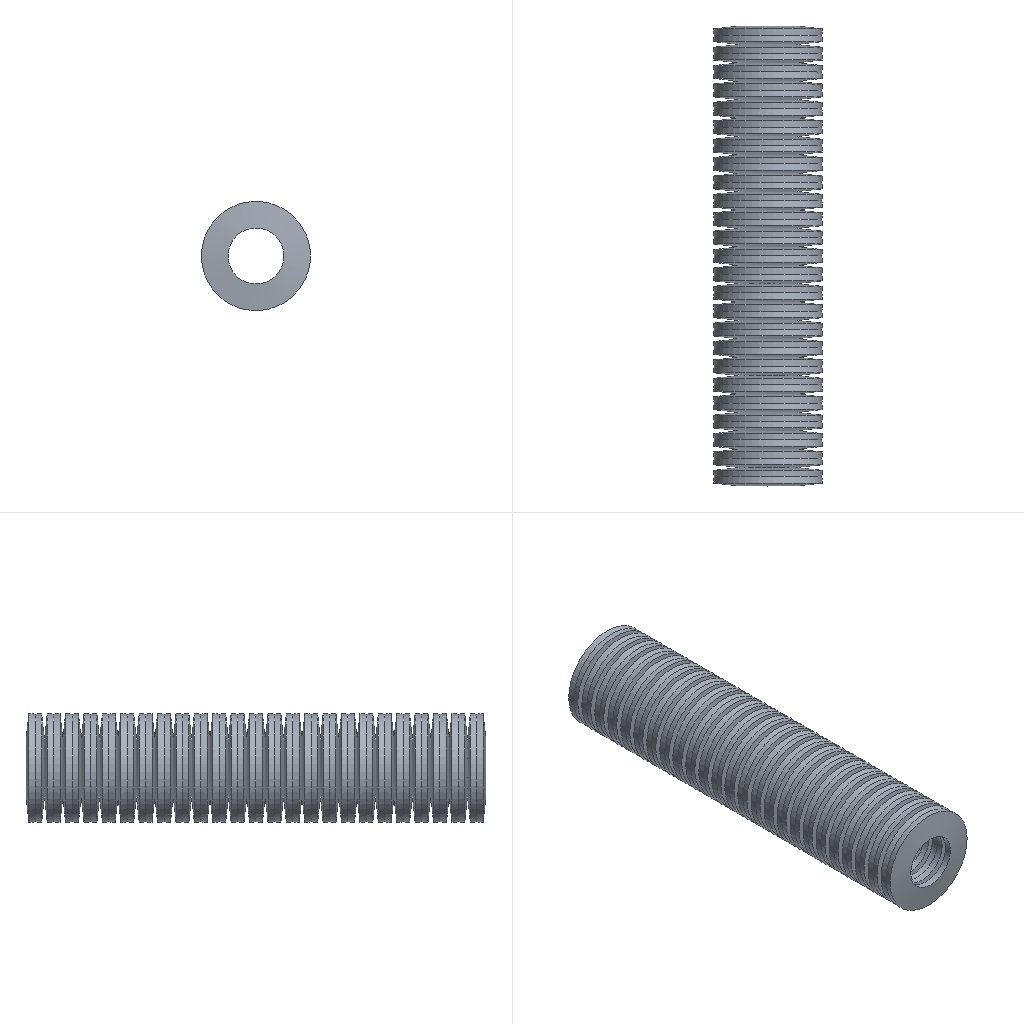Simulation study | abaqus
Set-up summary:
category,name,step,type,value,unit,region
solver,abaqus,,Abaqus/CAE 2024
units,mm-N-s-tonne (MPa),,inferred,E=206000 density=
analysis,Step-1,,static,time_period=0.24
mesh,nodes,,,129300
mesh,elements,,,18800
element_type,C3D20R,,,18800
material,Material-1,,E,206000
material,Material-1,,nu,0.3
section,Material-1,,solid section,,,_PickedSet2
bc,BC-1,initial,encastre,[dofs=ENCASTRE],,_PickedSet110
bc,BC-2,Step-1,fixed,"[dofs=rx,ry,rz,x,z n=5]",,_PickedSet113
bc,BC-2,Step-1,displacement,-1 [dofs=y],,_PickedSet113
contact,Int-1,initial,general contact,interaction=IntProp-3; friction=0.2; behavior=hard
constraint,coupling,,,1
Abaqus input file, long lists of numbers shortened, first 393 of 2027 lines:
*Heading
** Job name: deck Model name: Model-1
** Generated by: Abaqus/CAE 2024
*Preprint, echo=NO, model=NO, history=NO, contact=NO
**
** PARTS
**
*Part, name=Part-1
*Node
      1,          80.,   22.911,           0.
      2,   79.157,   13.549,           0.
** (2583 more lines like these left out)
*Element, type=C3D20R
  1,   31,   21,   17,   26,   15,    5,    1,   10,  756,  755,  754,  753,  757,  758,  759,
      760,  762,  761,  763,  764
** (750 more lines like these left out)
*Node
   2586,           0.,   27.049, 2.51052603e-15
*Nset, nset=Part-1-RefPt_, internal
2586,
*Nset, nset=_PickedSet2, internal, generate
    1,  2585,     1
*Elset, elset=_PickedSet2, internal, generate
   1,  376,    1
*Nset, nset=Set-1
    3,   19,   35,   51,   67,   83,   99,  115,  131,  147,  163,  179,  195,  211,  227,  243
  259,  275,  291,  307,  323,  339,  355,  371,  387,  403,  419,  435,  451,  467,  483,  499
** (4 more lines like these left out)
*Elset, elset=Set-1, generate
   4,  372,    8
** Section: Section-1
*Solid Section, elset=_PickedSet2, material=Material-1
,
*End Part
**
**
** ASSEMBLY
**
*Assembly, name=Assembly
**
*Instance, name=Part-1-1, part=Part-1
          0.,    -0.04861,           0.
*End Instance
**
*Instance, name=Part-1-2, part=Part-1
          0.,    27.049,           0.
          0.,    27.049,           0.,           1.,    27.049,           0.,         180.
*End Instance
**
*Instance, name=Part-1-1-lin-1-2, part=Part-1
          0.,    26.951,           0.
*End Instance
**
*Instance, name=Part-1-1-lin-1-3, part=Part-1
          0.,    53.951,           0.
*End Instance
**
*Instance, name=Part-1-1-lin-1-4, part=Part-1
          0.,    80.951,           0.
*End Instance
**
*Instance, name=Part-1-1-lin-1-5, part=Part-1
          0.,   107.951,           0.
*End Instance
**
*Instance, name=Part-1-1-lin-1-6, part=Part-1
          0.,   134.951,           0.
*End Instance
**
*Instance, name=Part-1-1-lin-1-7, part=Part-1
          0.,   161.951,           0.
*End Instance
**
*Instance, name=Part-1-1-lin-1-8, part=Part-1
          0.,   188.951,           0.
*End Instance
**
*Instance, name=Part-1-1-lin-1-9, part=Part-1
          0.,   215.951,           0.
*End Instance
**
*Instance, name=Part-1-1-lin-1-10, part=Part-1
          0.,   242.951,           0.
*End Instance
**
*Instance, name=Part-1-1-lin-1-11, part=Part-1
          0.,   269.951,           0.
*End Instance
**
*Instance, name=Part-1-1-lin-1-12, part=Part-1
          0.,   296.951,           0.
*End Instance
**
*Instance, name=Part-1-1-lin-1-13, part=Part-1
          0.,   323.951,           0.
*End Instance
**
*Instance, name=Part-1-1-lin-1-14, part=Part-1
          0.,   350.951,           0.
*End Instance
**
*Instance, name=Part-1-1-lin-1-15, part=Part-1
          0.,   377.951,           0.
*End Instance
**
*Instance, name=Part-1-1-lin-1-16, part=Part-1
          0.,   404.951,           0.
*End Instance
**
*Instance, name=Part-1-1-lin-1-17, part=Part-1
          0.,   431.951,           0.
*End Instance
**
*Instance, name=Part-1-1-lin-1-18, part=Part-1
          0.,   458.951,           0.
*End Instance
**
*Instance, name=Part-1-1-lin-1-19, part=Part-1
          0.,   485.951,           0.
*End Instance
**
*Instance, name=Part-1-1-lin-1-20, part=Part-1
          0.,   512.951,           0.
*End Instance
**
*Instance, name=Part-1-1-lin-1-21, part=Part-1
          0.,   539.951,           0.
*End Instance
**
*Instance, name=Part-1-1-lin-1-22, part=Part-1
          0.,   566.951,           0.
*End Instance
**
*Instance, name=Part-1-1-lin-1-23, part=Part-1
          0.,   593.951,           0.
*End Instance
**
*Instance, name=Part-1-1-lin-1-24, part=Part-1
          0.,   620.951,           0.
*End Instance
**
*Instance, name=Part-1-1-lin-1-25, part=Part-1
          0.,   647.951,           0.
*End Instance
**
*Instance, name=Part-1-2-lin-1-2, part=Part-1
          0.,    54.049,           0.
          0.,    54.049,           0.,           1.,    54.049,           0.,         180.
*End Instance
**
*Instance, name=Part-1-2-lin-1-3, part=Part-1
          0.,    81.049,           0.
          0.,    81.049,           0.,           1.,    81.049,           0.,         180.
*End Instance
**
*Instance, name=Part-1-2-lin-1-4, part=Part-1
          0.,   108.049,           0.
          0.,   108.049,           0.,           1.,   108.049,           0.,         180.
*End Instance
**
*Instance, name=Part-1-2-lin-1-5, part=Part-1
          0.,   135.049,           0.
          0.,   135.049,           0.,           1.,   135.049,           0.,         180.
*End Instance
**
*Instance, name=Part-1-2-lin-1-6, part=Part-1
          0.,   162.049,           0.
          0.,   162.049,           0.,           1.,   162.049,           0.,         180.
*End Instance
**
*Instance, name=Part-1-2-lin-1-7, part=Part-1
          0.,   189.049,           0.
          0.,   189.049,           0.,           1.,   189.049,           0.,         180.
*End Instance
**
*Instance, name=Part-1-2-lin-1-8, part=Part-1
          0.,   216.049,           0.
          0.,   216.049,           0.,           1.,   216.049,           0.,         180.
*End Instance
**
*Instance, name=Part-1-2-lin-1-9, part=Part-1
          0.,   243.049,           0.
          0.,   243.049,           0.,           1.,   243.049,           0.,         180.
*End Instance
**
*Instance, name=Part-1-2-lin-1-10, part=Part-1
          0.,   270.049,           0.
          0.,   270.049,           0.,           1.,   270.049,           0.,         180.
*End Instance
**
*Instance, name=Part-1-2-lin-1-11, part=Part-1
          0.,   297.049,           0.
          0.,   297.049,           0.,           1.,   297.049,           0.,         180.
*End Instance
**
*Instance, name=Part-1-2-lin-1-12, part=Part-1
          0.,   324.049,           0.
          0.,   324.049,           0.,           1.,   324.049,           0.,         180.
*End Instance
**
*Instance, name=Part-1-2-lin-1-13, part=Part-1
          0.,   351.049,           0.
          0.,   351.049,           0.,           1.,   351.049,           0.,         180.
*End Instance
**
*Instance, name=Part-1-2-lin-1-14, part=Part-1
          0.,   378.049,           0.
          0.,   378.049,           0.,           1.,   378.049,           0.,         180.
*End Instance
**
*Instance, name=Part-1-2-lin-1-15, part=Part-1
          0.,   405.049,           0.
          0.,   405.049,           0.,           1.,   405.049,           0.,         180.
*End Instance
**
*Instance, name=Part-1-2-lin-1-16, part=Part-1
          0.,   432.049,           0.
          0.,   432.049,           0.,           1.,   432.049,           0.,         180.
*End Instance
**
*Instance, name=Part-1-2-lin-1-17, part=Part-1
          0.,   459.049,           0.
          0.,   459.049,           0.,           1.,   459.049,           0.,         180.
*End Instance
**
*Instance, name=Part-1-2-lin-1-18, part=Part-1
          0.,   486.049,           0.
          0.,   486.049,           0.,           1.,   486.049,           0.,         180.
*End Instance
**
*Instance, name=Part-1-2-lin-1-19, part=Part-1
          0.,   513.049,           0.
          0.,   513.049,           0.,           1.,   513.049,           0.,         180.
*End Instance
**
*Instance, name=Part-1-2-lin-1-20, part=Part-1
          0.,   540.049,           0.
          0.,   540.049,           0.,           1.,   540.049,           0.,         180.
*End Instance
**
*Instance, name=Part-1-2-lin-1-21, part=Part-1
          0.,   567.049,           0.
          0.,   567.049,           0.,           1.,   567.049,           0.,         180.
*End Instance
**
*Instance, name=Part-1-2-lin-1-22, part=Part-1
          0.,   594.049,           0.
          0.,   594.049,           0.,           1.,   594.049,           0.,         180.
*End Instance
**
*Instance, name=Part-1-2-lin-1-23, part=Part-1
          0.,   621.049,           0.
          0.,   621.049,           0.,           1.,   621.049,           0.,         180.
*End Instance
**
*Instance, name=Part-1-2-lin-1-24, part=Part-1
          0.,   648.049,           0.
          0.,   648.049,           0.,           1.,   648.049,           0.,         180.
*End Instance
**
*Instance, name=Part-1-2-lin-1-25, part=Part-1
          0.,   675.049,           0.
          0.,   675.049,           0.,           1.,   675.049,           0.,         180.
*End Instance
**
*Nset, nset=Set-1, instance=Part-1-1-lin-1-25
 2586,
*Nset, nset=_PickedSet110, internal, instance=Part-1-2
    3,   19,   35,   51,   67,   83,   99,  115,  131,  147,  163,  179,  195,  211,  227,  243
  259,  275,  291,  307,  323,  339,  355,  371,  387,  403,  419,  435,  451,  467,  483,  499
** (4 more lines like these left out)
*Elset, elset=_PickedSet110, internal, instance=Part-1-2, generate
   4,  372,    8
*Nset, nset=_PickedSet113, internal, instance=Part-1-1-lin-1-25
 2586,
*Nset, nset=_PickedSet118, internal, instance=Part-1-2
    3,   19,   35,   51,   67,   83,   99,  115,  131,  147,  163,  179,  195,  211,  227,  243
  259,  275,  291,  307,  323,  339,  355,  371,  387,  403,  419,  435,  451,  467,  483,  499
** (4 more lines like these left out)
*Elset, elset=_PickedSet118, internal, instance=Part-1-2, generate
   4,  372,    8
*Nset, nset=_PickedSet119, internal, instance=Part-1-2
 2586,
*Nset, nset=_PickedSet120, internal, instance=Part-1-1-lin-1-25
    3,   19,   35,   51,   67,   83,   99,  115,  131,  147,  163,  179,  195,  211,  227,  243
  259,  275,  291,  307,  323,  339,  355,  371,  387,  403,  419,  435,  451,  467,  483,  499
** (4 more lines like these left out)
*Elset, elset=_PickedSet120, internal, instance=Part-1-1-lin-1-25, generate
   4,  372,    8
*Nset, nset=_PickedSet121, internal, instance=Part-1-1-lin-1-25
 2586,
*Surface, type=NODE, name=_PickedSet120_CNS_, internal
_PickedSet120, 1.
** Constraint: Constraint-2
*Coupling, constraint name=Constraint-2, ref node=_PickedSet121, surface=_PickedSet120_CNS_
*Kinematic
*Elset, elset=__Int-1_gcs0_1_S4, internal, instance=Part-1-1, generate
   1,  369,    8
*Elset, elset=__Int-1_gcs0_1_S5, internal, instance=Part-1-1, generate
   7,  375,    8
*Elset, elset=__Int-1_gcs0_1_S3, internal, instance=Part-1-1, generate
   8,  376,    8
*Surface, type=ELEMENT, name=_Int-1_gcs0_1, internal
__Int-1_gcs0_1_S4, S4
__Int-1_gcs0_1_S5, S5
__Int-1_gcs0_1_S3, S3
*Elset, elset=__Int-1_gcs0_2_S5, internal, instance=Part-1-1
   2,   4,   5,   6,  10,  12,  13,  14,  18,  20,  21,  22,  26,  28,  29,  30
  34,  36,  37,  38,  42,  44,  45,  46,  50,  52,  53,  54,  58,  60,  61,  62
** (10 more lines like these left out)
*Elset, elset=__Int-1_gcs0_2_S6, internal, instance=Part-1-1, generate
   8,  376,    8
*Surface, type=ELEMENT, name=_Int-1_gcs0_2, internal
__Int-1_gcs0_2_S5, S5
__Int-1_gcs0_2_S6, S6
*Elset, elset=__Int-1_gcs0_3_S4, internal, instance=Part-1-1, generate
   4,  372,    8
*Surface, type=ELEMENT, name=_Int-1_gcs0_3, internal
__Int-1_gcs0_3_S4, S4
*Elset, elset=__Int-1_gcs0_4_S5, internal, instance=Part-1-1, generate
   1,  369,    8
*Elset, elset=__Int-1_gcs0_4_S3, internal, instance=Part-1-1
   2,   4,   5,   6,  10,  12,  13,  14,  18,  20,  21,  22,  26,  28,  29,  30
  34,  36,  37,  38,  42,  44,  45,  46,  50,  52,  53,  54,  58,  60,  61,  62
** (10 more lines like these left out)
*Surface, type=ELEMENT, name=_Int-1_gcs0_4, internal
__Int-1_gcs0_4_S5, S5
__Int-1_gcs0_4_S3, S3
*Elset, elset=__Int-1_gcs0_5_S4, internal, instance=Part-1-2, generate
   1,  369,    8
*Elset, elset=__Int-1_gcs0_5_S5, internal, instance=Part-1-2, generate
   7,  375,    8
*Elset, elset=__Int-1_gcs0_5_S3, internal, instance=Part-1-2, generate
   8,  376,    8
*Surface, type=ELEMENT, name=_Int-1_gcs0_5, internal
__Int-1_gcs0_5_S4, S4
__Int-1_gcs0_5_S5, S5
__Int-1_gcs0_5_S3, S3
*Elset, elset=__Int-1_gcs0_6_S5, internal, instance=Part-1-2
   2,   4,   5,   6,  10,  12,  13,  14,  18,  20,  21,  22,  26,  28,  29,  30
  34,  36,  37,  38,  42,  44,  45,  46,  50,  52,  53,  54,  58,  60,  61,  62
** (10 more lines like these left out)
*Elset, elset=__Int-1_gcs0_6_S6, internal, instance=Part-1-2, generate
   8,  376,    8
*Surface, type=ELEMENT, name=_Int-1_gcs0_6, internal
__Int-1_gcs0_6_S5, S5
__Int-1_gcs0_6_S6, S6
*Elset, elset=__Int-1_gcs0_7_S4, internal, instance=Part-1-2, generate
   4,  372,    8
*Surface, type=ELEMENT, name=_Int-1_gcs0_7, internal
__Int-1_gcs0_7_S4, S4
*Elset, elset=__Int-1_gcs0_8_S5, internal, instance=Part-1-2, generate
   1,  369,    8
*Elset, elset=__Int-1_gcs0_8_S3, internal, instance=Part-1-2
   2,   4,   5,   6,  10,  12,  13,  14,  18,  20,  21,  22,  26,  28,  29,  30
  34,  36,  37,  38,  42,  44,  45,  46,  50,  52,  53,  54,  58,  60,  61,  62
** (10 more lines like these left out)
*Surface, type=ELEMENT, name=_Int-1_gcs0_8, internal
__Int-1_gcs0_8_S5, S5
__Int-1_gcs0_8_S3, S3
*Elset, elset=__Int-1_gcs0_9_S4, internal, instance=Part-1-1-lin-1-2, generate
   1,  369,    8
*Elset, elset=__Int-1_gcs0_9_S5, internal, instance=Part-1-1-lin-1-2, generate
   7,  375,    8
*Elset, elset=__Int-1_gcs0_9_S3, internal, instance=Part-1-1-lin-1-2, generate
   8,  376,    8
*Surface, type=ELEMENT, name=_Int-1_gcs0_9, internal
__Int-1_gcs0_9_S4, S4
__Int-1_gcs0_9_S5, S5
__Int-1_gcs0_9_S3, S3
*Elset, elset=__Int-1_gcs0_10_S5, internal, instance=Part-1-1-lin-1-2
   2,   4,   5,   6,  10,  12,  13,  14,  18,  20,  21,  22,  26,  28,  29,  30
  34,  36,  37,  38,  42,  44,  45,  46,  50,  52,  53,  54,  58,  60,  61,  62
** (10 more lines like these left out)
*Elset, elset=__Int-1_gcs0_10_S6, internal, instance=Part-1-1-lin-1-2, generate
   8,  376,    8
*Surface, type=ELEMENT, name=_Int-1_gcs0_10, internal
__Int-1_gcs0_10_S5, S5
__Int-1_gcs0_10_S6, S6
*Elset, elset=__Int-1_gcs0_11_S4, internal, instance=Part-1-1-lin-1-2, generate
   4,  372,    8
*Surface, type=ELEMENT, name=_Int-1_gcs0_11, internal
__Int-1_gcs0_11_S4, S4
*Elset, elset=__Int-1_gcs0_12_S5, internal, instance=Part-1-1-lin-1-2, generate
   1,  369,    8
*Elset, elset=__Int-1_gcs0_12_S3, internal, instance=Part-1-1-lin-1-2
   2,   4,   5,   6,  10,  12,  13,  14,  18,  20,  21,  22,  26,  28,  29,  30
  34,  36,  37,  38,  42,  44,  45,  46,  50,  52,  53,  54,  58,  60,  61,  62
** (10 more lines like these left out)
*Surface, type=ELEMENT, name=_Int-1_gcs0_12, internal
__Int-1_gcs0_12_S5, S5
__Int-1_gcs0_12_S3, S3
*Elset, elset=__Int-1_gcs0_13_S4, internal, instance=Part-1-1-lin-1-3, generate
Last 640 lines:
   7,  375,    8
*Elset, elset=__Int-1_gcs0_137_S3, internal, instance=Part-1-2-lin-1-10, generate
   8,  376,    8
*Surface, type=ELEMENT, name=_Int-1_gcs0_137, internal
__Int-1_gcs0_137_S4, S4
__Int-1_gcs0_137_S5, S5
__Int-1_gcs0_137_S3, S3
*Elset, elset=__Int-1_gcs0_138_S5, internal, instance=Part-1-2-lin-1-10
   2,   4,   5,   6,  10,  12,  13,  14,  18,  20,  21,  22,  26,  28,  29,  30
  34,  36,  37,  38,  42,  44,  45,  46,  50,  52,  53,  54,  58,  60,  61,  62
** (10 more lines like these left out)
*Elset, elset=__Int-1_gcs0_138_S6, internal, instance=Part-1-2-lin-1-10, generate
   8,  376,    8
*Surface, type=ELEMENT, name=_Int-1_gcs0_138, internal
__Int-1_gcs0_138_S5, S5
__Int-1_gcs0_138_S6, S6
*Elset, elset=__Int-1_gcs0_139_S4, internal, instance=Part-1-2-lin-1-10, generate
   4,  372,    8
*Surface, type=ELEMENT, name=_Int-1_gcs0_139, internal
__Int-1_gcs0_139_S4, S4
*Elset, elset=__Int-1_gcs0_140_S5, internal, instance=Part-1-2-lin-1-10, generate
   1,  369,    8
*Elset, elset=__Int-1_gcs0_140_S3, internal, instance=Part-1-2-lin-1-10
   2,   4,   5,   6,  10,  12,  13,  14,  18,  20,  21,  22,  26,  28,  29,  30
  34,  36,  37,  38,  42,  44,  45,  46,  50,  52,  53,  54,  58,  60,  61,  62
** (10 more lines like these left out)
*Surface, type=ELEMENT, name=_Int-1_gcs0_140, internal
__Int-1_gcs0_140_S5, S5
__Int-1_gcs0_140_S3, S3
*Elset, elset=__Int-1_gcs0_141_S4, internal, instance=Part-1-2-lin-1-11, generate
   1,  369,    8
*Elset, elset=__Int-1_gcs0_141_S5, internal, instance=Part-1-2-lin-1-11, generate
   7,  375,    8
*Elset, elset=__Int-1_gcs0_141_S3, internal, instance=Part-1-2-lin-1-11, generate
   8,  376,    8
*Surface, type=ELEMENT, name=_Int-1_gcs0_141, internal
__Int-1_gcs0_141_S4, S4
__Int-1_gcs0_141_S5, S5
__Int-1_gcs0_141_S3, S3
*Elset, elset=__Int-1_gcs0_142_S5, internal, instance=Part-1-2-lin-1-11
   2,   4,   5,   6,  10,  12,  13,  14,  18,  20,  21,  22,  26,  28,  29,  30
  34,  36,  37,  38,  42,  44,  45,  46,  50,  52,  53,  54,  58,  60,  61,  62
** (10 more lines like these left out)
*Elset, elset=__Int-1_gcs0_142_S6, internal, instance=Part-1-2-lin-1-11, generate
   8,  376,    8
*Surface, type=ELEMENT, name=_Int-1_gcs0_142, internal
__Int-1_gcs0_142_S5, S5
__Int-1_gcs0_142_S6, S6
*Elset, elset=__Int-1_gcs0_143_S4, internal, instance=Part-1-2-lin-1-11, generate
   4,  372,    8
*Surface, type=ELEMENT, name=_Int-1_gcs0_143, internal
__Int-1_gcs0_143_S4, S4
*Elset, elset=__Int-1_gcs0_144_S5, internal, instance=Part-1-2-lin-1-11, generate
   1,  369,    8
*Elset, elset=__Int-1_gcs0_144_S3, internal, instance=Part-1-2-lin-1-11
   2,   4,   5,   6,  10,  12,  13,  14,  18,  20,  21,  22,  26,  28,  29,  30
  34,  36,  37,  38,  42,  44,  45,  46,  50,  52,  53,  54,  58,  60,  61,  62
** (10 more lines like these left out)
*Surface, type=ELEMENT, name=_Int-1_gcs0_144, internal
__Int-1_gcs0_144_S5, S5
__Int-1_gcs0_144_S3, S3
*Elset, elset=__Int-1_gcs0_145_S4, internal, instance=Part-1-2-lin-1-12, generate
   1,  369,    8
*Elset, elset=__Int-1_gcs0_145_S5, internal, instance=Part-1-2-lin-1-12, generate
   7,  375,    8
*Elset, elset=__Int-1_gcs0_145_S3, internal, instance=Part-1-2-lin-1-12, generate
   8,  376,    8
*Surface, type=ELEMENT, name=_Int-1_gcs0_145, internal
__Int-1_gcs0_145_S4, S4
__Int-1_gcs0_145_S5, S5
__Int-1_gcs0_145_S3, S3
*Elset, elset=__Int-1_gcs0_146_S5, internal, instance=Part-1-2-lin-1-12
   2,   4,   5,   6,  10,  12,  13,  14,  18,  20,  21,  22,  26,  28,  29,  30
  34,  36,  37,  38,  42,  44,  45,  46,  50,  52,  53,  54,  58,  60,  61,  62
** (10 more lines like these left out)
*Elset, elset=__Int-1_gcs0_146_S6, internal, instance=Part-1-2-lin-1-12, generate
   8,  376,    8
*Surface, type=ELEMENT, name=_Int-1_gcs0_146, internal
__Int-1_gcs0_146_S5, S5
__Int-1_gcs0_146_S6, S6
*Elset, elset=__Int-1_gcs0_147_S4, internal, instance=Part-1-2-lin-1-12, generate
   4,  372,    8
*Surface, type=ELEMENT, name=_Int-1_gcs0_147, internal
__Int-1_gcs0_147_S4, S4
*Elset, elset=__Int-1_gcs0_148_S5, internal, instance=Part-1-2-lin-1-12, generate
   1,  369,    8
*Elset, elset=__Int-1_gcs0_148_S3, internal, instance=Part-1-2-lin-1-12
   2,   4,   5,   6,  10,  12,  13,  14,  18,  20,  21,  22,  26,  28,  29,  30
  34,  36,  37,  38,  42,  44,  45,  46,  50,  52,  53,  54,  58,  60,  61,  62
** (10 more lines like these left out)
*Surface, type=ELEMENT, name=_Int-1_gcs0_148, internal
__Int-1_gcs0_148_S5, S5
__Int-1_gcs0_148_S3, S3
*Elset, elset=__Int-1_gcs0_149_S4, internal, instance=Part-1-2-lin-1-13, generate
   1,  369,    8
*Elset, elset=__Int-1_gcs0_149_S5, internal, instance=Part-1-2-lin-1-13, generate
   7,  375,    8
*Elset, elset=__Int-1_gcs0_149_S3, internal, instance=Part-1-2-lin-1-13, generate
   8,  376,    8
*Surface, type=ELEMENT, name=_Int-1_gcs0_149, internal
__Int-1_gcs0_149_S4, S4
__Int-1_gcs0_149_S5, S5
__Int-1_gcs0_149_S3, S3
*Elset, elset=__Int-1_gcs0_150_S5, internal, instance=Part-1-2-lin-1-13
   2,   4,   5,   6,  10,  12,  13,  14,  18,  20,  21,  22,  26,  28,  29,  30
  34,  36,  37,  38,  42,  44,  45,  46,  50,  52,  53,  54,  58,  60,  61,  62
** (10 more lines like these left out)
*Elset, elset=__Int-1_gcs0_150_S6, internal, instance=Part-1-2-lin-1-13, generate
   8,  376,    8
*Surface, type=ELEMENT, name=_Int-1_gcs0_150, internal
__Int-1_gcs0_150_S5, S5
__Int-1_gcs0_150_S6, S6
*Elset, elset=__Int-1_gcs0_151_S4, internal, instance=Part-1-2-lin-1-13, generate
   4,  372,    8
*Surface, type=ELEMENT, name=_Int-1_gcs0_151, internal
__Int-1_gcs0_151_S4, S4
*Elset, elset=__Int-1_gcs0_152_S5, internal, instance=Part-1-2-lin-1-13, generate
   1,  369,    8
*Elset, elset=__Int-1_gcs0_152_S3, internal, instance=Part-1-2-lin-1-13
   2,   4,   5,   6,  10,  12,  13,  14,  18,  20,  21,  22,  26,  28,  29,  30
  34,  36,  37,  38,  42,  44,  45,  46,  50,  52,  53,  54,  58,  60,  61,  62
** (10 more lines like these left out)
*Surface, type=ELEMENT, name=_Int-1_gcs0_152, internal
__Int-1_gcs0_152_S5, S5
__Int-1_gcs0_152_S3, S3
*Elset, elset=__Int-1_gcs0_153_S4, internal, instance=Part-1-2-lin-1-14, generate
   1,  369,    8
*Elset, elset=__Int-1_gcs0_153_S5, internal, instance=Part-1-2-lin-1-14, generate
   7,  375,    8
*Elset, elset=__Int-1_gcs0_153_S3, internal, instance=Part-1-2-lin-1-14, generate
   8,  376,    8
*Surface, type=ELEMENT, name=_Int-1_gcs0_153, internal
__Int-1_gcs0_153_S4, S4
__Int-1_gcs0_153_S5, S5
__Int-1_gcs0_153_S3, S3
*Elset, elset=__Int-1_gcs0_154_S5, internal, instance=Part-1-2-lin-1-14
   2,   4,   5,   6,  10,  12,  13,  14,  18,  20,  21,  22,  26,  28,  29,  30
  34,  36,  37,  38,  42,  44,  45,  46,  50,  52,  53,  54,  58,  60,  61,  62
** (10 more lines like these left out)
*Elset, elset=__Int-1_gcs0_154_S6, internal, instance=Part-1-2-lin-1-14, generate
   8,  376,    8
*Surface, type=ELEMENT, name=_Int-1_gcs0_154, internal
__Int-1_gcs0_154_S5, S5
__Int-1_gcs0_154_S6, S6
*Elset, elset=__Int-1_gcs0_155_S4, internal, instance=Part-1-2-lin-1-14, generate
   4,  372,    8
*Surface, type=ELEMENT, name=_Int-1_gcs0_155, internal
__Int-1_gcs0_155_S4, S4
*Elset, elset=__Int-1_gcs0_156_S5, internal, instance=Part-1-2-lin-1-14, generate
   1,  369,    8
*Elset, elset=__Int-1_gcs0_156_S3, internal, instance=Part-1-2-lin-1-14
   2,   4,   5,   6,  10,  12,  13,  14,  18,  20,  21,  22,  26,  28,  29,  30
  34,  36,  37,  38,  42,  44,  45,  46,  50,  52,  53,  54,  58,  60,  61,  62
** (10 more lines like these left out)
*Surface, type=ELEMENT, name=_Int-1_gcs0_156, internal
__Int-1_gcs0_156_S5, S5
__Int-1_gcs0_156_S3, S3
*Elset, elset=__Int-1_gcs0_157_S4, internal, instance=Part-1-2-lin-1-15, generate
   1,  369,    8
*Elset, elset=__Int-1_gcs0_157_S5, internal, instance=Part-1-2-lin-1-15, generate
   7,  375,    8
*Elset, elset=__Int-1_gcs0_157_S3, internal, instance=Part-1-2-lin-1-15, generate
   8,  376,    8
*Surface, type=ELEMENT, name=_Int-1_gcs0_157, internal
__Int-1_gcs0_157_S4, S4
__Int-1_gcs0_157_S5, S5
__Int-1_gcs0_157_S3, S3
*Elset, elset=__Int-1_gcs0_158_S5, internal, instance=Part-1-2-lin-1-15
   2,   4,   5,   6,  10,  12,  13,  14,  18,  20,  21,  22,  26,  28,  29,  30
  34,  36,  37,  38,  42,  44,  45,  46,  50,  52,  53,  54,  58,  60,  61,  62
** (10 more lines like these left out)
*Elset, elset=__Int-1_gcs0_158_S6, internal, instance=Part-1-2-lin-1-15, generate
   8,  376,    8
*Surface, type=ELEMENT, name=_Int-1_gcs0_158, internal
__Int-1_gcs0_158_S5, S5
__Int-1_gcs0_158_S6, S6
*Elset, elset=__Int-1_gcs0_159_S4, internal, instance=Part-1-2-lin-1-15, generate
   4,  372,    8
*Surface, type=ELEMENT, name=_Int-1_gcs0_159, internal
__Int-1_gcs0_159_S4, S4
*Elset, elset=__Int-1_gcs0_160_S5, internal, instance=Part-1-2-lin-1-15, generate
   1,  369,    8
*Elset, elset=__Int-1_gcs0_160_S3, internal, instance=Part-1-2-lin-1-15
   2,   4,   5,   6,  10,  12,  13,  14,  18,  20,  21,  22,  26,  28,  29,  30
  34,  36,  37,  38,  42,  44,  45,  46,  50,  52,  53,  54,  58,  60,  61,  62
** (10 more lines like these left out)
*Surface, type=ELEMENT, name=_Int-1_gcs0_160, internal
__Int-1_gcs0_160_S5, S5
__Int-1_gcs0_160_S3, S3
*Elset, elset=__Int-1_gcs0_161_S4, internal, instance=Part-1-2-lin-1-16, generate
   1,  369,    8
*Elset, elset=__Int-1_gcs0_161_S5, internal, instance=Part-1-2-lin-1-16, generate
   7,  375,    8
*Elset, elset=__Int-1_gcs0_161_S3, internal, instance=Part-1-2-lin-1-16, generate
   8,  376,    8
*Surface, type=ELEMENT, name=_Int-1_gcs0_161, internal
__Int-1_gcs0_161_S4, S4
__Int-1_gcs0_161_S5, S5
__Int-1_gcs0_161_S3, S3
*Elset, elset=__Int-1_gcs0_162_S5, internal, instance=Part-1-2-lin-1-16
   2,   4,   5,   6,  10,  12,  13,  14,  18,  20,  21,  22,  26,  28,  29,  30
  34,  36,  37,  38,  42,  44,  45,  46,  50,  52,  53,  54,  58,  60,  61,  62
** (10 more lines like these left out)
*Elset, elset=__Int-1_gcs0_162_S6, internal, instance=Part-1-2-lin-1-16, generate
   8,  376,    8
*Surface, type=ELEMENT, name=_Int-1_gcs0_162, internal
__Int-1_gcs0_162_S5, S5
__Int-1_gcs0_162_S6, S6
*Elset, elset=__Int-1_gcs0_163_S4, internal, instance=Part-1-2-lin-1-16, generate
   4,  372,    8
*Surface, type=ELEMENT, name=_Int-1_gcs0_163, internal
__Int-1_gcs0_163_S4, S4
*Elset, elset=__Int-1_gcs0_164_S5, internal, instance=Part-1-2-lin-1-16, generate
   1,  369,    8
*Elset, elset=__Int-1_gcs0_164_S3, internal, instance=Part-1-2-lin-1-16
   2,   4,   5,   6,  10,  12,  13,  14,  18,  20,  21,  22,  26,  28,  29,  30
  34,  36,  37,  38,  42,  44,  45,  46,  50,  52,  53,  54,  58,  60,  61,  62
** (10 more lines like these left out)
*Surface, type=ELEMENT, name=_Int-1_gcs0_164, internal
__Int-1_gcs0_164_S5, S5
__Int-1_gcs0_164_S3, S3
*Elset, elset=__Int-1_gcs0_165_S4, internal, instance=Part-1-2-lin-1-17, generate
   1,  369,    8
*Elset, elset=__Int-1_gcs0_165_S5, internal, instance=Part-1-2-lin-1-17, generate
   7,  375,    8
*Elset, elset=__Int-1_gcs0_165_S3, internal, instance=Part-1-2-lin-1-17, generate
   8,  376,    8
*Surface, type=ELEMENT, name=_Int-1_gcs0_165, internal
__Int-1_gcs0_165_S4, S4
__Int-1_gcs0_165_S5, S5
__Int-1_gcs0_165_S3, S3
*Elset, elset=__Int-1_gcs0_166_S5, internal, instance=Part-1-2-lin-1-17
   2,   4,   5,   6,  10,  12,  13,  14,  18,  20,  21,  22,  26,  28,  29,  30
  34,  36,  37,  38,  42,  44,  45,  46,  50,  52,  53,  54,  58,  60,  61,  62
** (10 more lines like these left out)
*Elset, elset=__Int-1_gcs0_166_S6, internal, instance=Part-1-2-lin-1-17, generate
   8,  376,    8
*Surface, type=ELEMENT, name=_Int-1_gcs0_166, internal
__Int-1_gcs0_166_S5, S5
__Int-1_gcs0_166_S6, S6
*Elset, elset=__Int-1_gcs0_167_S4, internal, instance=Part-1-2-lin-1-17, generate
   4,  372,    8
*Surface, type=ELEMENT, name=_Int-1_gcs0_167, internal
__Int-1_gcs0_167_S4, S4
*Elset, elset=__Int-1_gcs0_168_S5, internal, instance=Part-1-2-lin-1-17, generate
   1,  369,    8
*Elset, elset=__Int-1_gcs0_168_S3, internal, instance=Part-1-2-lin-1-17
   2,   4,   5,   6,  10,  12,  13,  14,  18,  20,  21,  22,  26,  28,  29,  30
  34,  36,  37,  38,  42,  44,  45,  46,  50,  52,  53,  54,  58,  60,  61,  62
** (10 more lines like these left out)
*Surface, type=ELEMENT, name=_Int-1_gcs0_168, internal
__Int-1_gcs0_168_S5, S5
__Int-1_gcs0_168_S3, S3
*Elset, elset=__Int-1_gcs0_169_S4, internal, instance=Part-1-2-lin-1-18, generate
   1,  369,    8
*Elset, elset=__Int-1_gcs0_169_S5, internal, instance=Part-1-2-lin-1-18, generate
   7,  375,    8
*Elset, elset=__Int-1_gcs0_169_S3, internal, instance=Part-1-2-lin-1-18, generate
   8,  376,    8
*Surface, type=ELEMENT, name=_Int-1_gcs0_169, internal
__Int-1_gcs0_169_S4, S4
__Int-1_gcs0_169_S5, S5
__Int-1_gcs0_169_S3, S3
*Elset, elset=__Int-1_gcs0_170_S5, internal, instance=Part-1-2-lin-1-18
   2,   4,   5,   6,  10,  12,  13,  14,  18,  20,  21,  22,  26,  28,  29,  30
  34,  36,  37,  38,  42,  44,  45,  46,  50,  52,  53,  54,  58,  60,  61,  62
** (10 more lines like these left out)
*Elset, elset=__Int-1_gcs0_170_S6, internal, instance=Part-1-2-lin-1-18, generate
   8,  376,    8
*Surface, type=ELEMENT, name=_Int-1_gcs0_170, internal
__Int-1_gcs0_170_S5, S5
__Int-1_gcs0_170_S6, S6
*Elset, elset=__Int-1_gcs0_171_S4, internal, instance=Part-1-2-lin-1-18, generate
   4,  372,    8
*Surface, type=ELEMENT, name=_Int-1_gcs0_171, internal
__Int-1_gcs0_171_S4, S4
*Elset, elset=__Int-1_gcs0_172_S5, internal, instance=Part-1-2-lin-1-18, generate
   1,  369,    8
*Elset, elset=__Int-1_gcs0_172_S3, internal, instance=Part-1-2-lin-1-18
   2,   4,   5,   6,  10,  12,  13,  14,  18,  20,  21,  22,  26,  28,  29,  30
  34,  36,  37,  38,  42,  44,  45,  46,  50,  52,  53,  54,  58,  60,  61,  62
** (10 more lines like these left out)
*Surface, type=ELEMENT, name=_Int-1_gcs0_172, internal
__Int-1_gcs0_172_S5, S5
__Int-1_gcs0_172_S3, S3
*Elset, elset=__Int-1_gcs0_173_S4, internal, instance=Part-1-2-lin-1-19, generate
   1,  369,    8
*Elset, elset=__Int-1_gcs0_173_S5, internal, instance=Part-1-2-lin-1-19, generate
   7,  375,    8
*Elset, elset=__Int-1_gcs0_173_S3, internal, instance=Part-1-2-lin-1-19, generate
   8,  376,    8
*Surface, type=ELEMENT, name=_Int-1_gcs0_173, internal
__Int-1_gcs0_173_S4, S4
__Int-1_gcs0_173_S5, S5
__Int-1_gcs0_173_S3, S3
*Elset, elset=__Int-1_gcs0_174_S5, internal, instance=Part-1-2-lin-1-19
   2,   4,   5,   6,  10,  12,  13,  14,  18,  20,  21,  22,  26,  28,  29,  30
  34,  36,  37,  38,  42,  44,  45,  46,  50,  52,  53,  54,  58,  60,  61,  62
** (10 more lines like these left out)
*Elset, elset=__Int-1_gcs0_174_S6, internal, instance=Part-1-2-lin-1-19, generate
   8,  376,    8
*Surface, type=ELEMENT, name=_Int-1_gcs0_174, internal
__Int-1_gcs0_174_S5, S5
__Int-1_gcs0_174_S6, S6
*Elset, elset=__Int-1_gcs0_175_S4, internal, instance=Part-1-2-lin-1-19, generate
   4,  372,    8
*Surface, type=ELEMENT, name=_Int-1_gcs0_175, internal
__Int-1_gcs0_175_S4, S4
*Elset, elset=__Int-1_gcs0_176_S5, internal, instance=Part-1-2-lin-1-19, generate
   1,  369,    8
*Elset, elset=__Int-1_gcs0_176_S3, internal, instance=Part-1-2-lin-1-19
   2,   4,   5,   6,  10,  12,  13,  14,  18,  20,  21,  22,  26,  28,  29,  30
  34,  36,  37,  38,  42,  44,  45,  46,  50,  52,  53,  54,  58,  60,  61,  62
** (10 more lines like these left out)
*Surface, type=ELEMENT, name=_Int-1_gcs0_176, internal
__Int-1_gcs0_176_S5, S5
__Int-1_gcs0_176_S3, S3
*Elset, elset=__Int-1_gcs0_177_S4, internal, instance=Part-1-2-lin-1-20, generate
   1,  369,    8
*Elset, elset=__Int-1_gcs0_177_S5, internal, instance=Part-1-2-lin-1-20, generate
   7,  375,    8
*Elset, elset=__Int-1_gcs0_177_S3, internal, instance=Part-1-2-lin-1-20, generate
   8,  376,    8
*Surface, type=ELEMENT, name=_Int-1_gcs0_177, internal
__Int-1_gcs0_177_S4, S4
__Int-1_gcs0_177_S5, S5
__Int-1_gcs0_177_S3, S3
*Elset, elset=__Int-1_gcs0_178_S5, internal, instance=Part-1-2-lin-1-20
   2,   4,   5,   6,  10,  12,  13,  14,  18,  20,  21,  22,  26,  28,  29,  30
  34,  36,  37,  38,  42,  44,  45,  46,  50,  52,  53,  54,  58,  60,  61,  62
** (10 more lines like these left out)
*Elset, elset=__Int-1_gcs0_178_S6, internal, instance=Part-1-2-lin-1-20, generate
   8,  376,    8
*Surface, type=ELEMENT, name=_Int-1_gcs0_178, internal
__Int-1_gcs0_178_S5, S5
__Int-1_gcs0_178_S6, S6
*Elset, elset=__Int-1_gcs0_179_S4, internal, instance=Part-1-2-lin-1-20, generate
   4,  372,    8
*Surface, type=ELEMENT, name=_Int-1_gcs0_179, internal
__Int-1_gcs0_179_S4, S4
*Elset, elset=__Int-1_gcs0_180_S5, internal, instance=Part-1-2-lin-1-20, generate
   1,  369,    8
*Elset, elset=__Int-1_gcs0_180_S3, internal, instance=Part-1-2-lin-1-20
   2,   4,   5,   6,  10,  12,  13,  14,  18,  20,  21,  22,  26,  28,  29,  30
  34,  36,  37,  38,  42,  44,  45,  46,  50,  52,  53,  54,  58,  60,  61,  62
** (10 more lines like these left out)
*Surface, type=ELEMENT, name=_Int-1_gcs0_180, internal
__Int-1_gcs0_180_S5, S5
__Int-1_gcs0_180_S3, S3
*Elset, elset=__Int-1_gcs0_181_S4, internal, instance=Part-1-2-lin-1-21, generate
   1,  369,    8
*Elset, elset=__Int-1_gcs0_181_S5, internal, instance=Part-1-2-lin-1-21, generate
   7,  375,    8
*Elset, elset=__Int-1_gcs0_181_S3, internal, instance=Part-1-2-lin-1-21, generate
   8,  376,    8
*Surface, type=ELEMENT, name=_Int-1_gcs0_181, internal
__Int-1_gcs0_181_S4, S4
__Int-1_gcs0_181_S5, S5
__Int-1_gcs0_181_S3, S3
*Elset, elset=__Int-1_gcs0_182_S5, internal, instance=Part-1-2-lin-1-21
   2,   4,   5,   6,  10,  12,  13,  14,  18,  20,  21,  22,  26,  28,  29,  30
  34,  36,  37,  38,  42,  44,  45,  46,  50,  52,  53,  54,  58,  60,  61,  62
** (10 more lines like these left out)
*Elset, elset=__Int-1_gcs0_182_S6, internal, instance=Part-1-2-lin-1-21, generate
   8,  376,    8
*Surface, type=ELEMENT, name=_Int-1_gcs0_182, internal
__Int-1_gcs0_182_S5, S5
__Int-1_gcs0_182_S6, S6
*Elset, elset=__Int-1_gcs0_183_S4, internal, instance=Part-1-2-lin-1-21, generate
   4,  372,    8
*Surface, type=ELEMENT, name=_Int-1_gcs0_183, internal
__Int-1_gcs0_183_S4, S4
*Elset, elset=__Int-1_gcs0_184_S5, internal, instance=Part-1-2-lin-1-21, generate
   1,  369,    8
*Elset, elset=__Int-1_gcs0_184_S3, internal, instance=Part-1-2-lin-1-21
   2,   4,   5,   6,  10,  12,  13,  14,  18,  20,  21,  22,  26,  28,  29,  30
  34,  36,  37,  38,  42,  44,  45,  46,  50,  52,  53,  54,  58,  60,  61,  62
** (10 more lines like these left out)
*Surface, type=ELEMENT, name=_Int-1_gcs0_184, internal
__Int-1_gcs0_184_S5, S5
__Int-1_gcs0_184_S3, S3
*Elset, elset=__Int-1_gcs0_185_S4, internal, instance=Part-1-2-lin-1-22, generate
   1,  369,    8
*Elset, elset=__Int-1_gcs0_185_S5, internal, instance=Part-1-2-lin-1-22, generate
   7,  375,    8
*Elset, elset=__Int-1_gcs0_185_S3, internal, instance=Part-1-2-lin-1-22, generate
   8,  376,    8
*Surface, type=ELEMENT, name=_Int-1_gcs0_185, internal
__Int-1_gcs0_185_S4, S4
__Int-1_gcs0_185_S5, S5
__Int-1_gcs0_185_S3, S3
*Elset, elset=__Int-1_gcs0_186_S5, internal, instance=Part-1-2-lin-1-22
   2,   4,   5,   6,  10,  12,  13,  14,  18,  20,  21,  22,  26,  28,  29,  30
  34,  36,  37,  38,  42,  44,  45,  46,  50,  52,  53,  54,  58,  60,  61,  62
** (10 more lines like these left out)
*Elset, elset=__Int-1_gcs0_186_S6, internal, instance=Part-1-2-lin-1-22, generate
   8,  376,    8
*Surface, type=ELEMENT, name=_Int-1_gcs0_186, internal
__Int-1_gcs0_186_S5, S5
__Int-1_gcs0_186_S6, S6
*Elset, elset=__Int-1_gcs0_187_S4, internal, instance=Part-1-2-lin-1-22, generate
   4,  372,    8
*Surface, type=ELEMENT, name=_Int-1_gcs0_187, internal
__Int-1_gcs0_187_S4, S4
*Elset, elset=__Int-1_gcs0_188_S5, internal, instance=Part-1-2-lin-1-22, generate
   1,  369,    8
*Elset, elset=__Int-1_gcs0_188_S3, internal, instance=Part-1-2-lin-1-22
   2,   4,   5,   6,  10,  12,  13,  14,  18,  20,  21,  22,  26,  28,  29,  30
  34,  36,  37,  38,  42,  44,  45,  46,  50,  52,  53,  54,  58,  60,  61,  62
** (10 more lines like these left out)
*Surface, type=ELEMENT, name=_Int-1_gcs0_188, internal
__Int-1_gcs0_188_S5, S5
__Int-1_gcs0_188_S3, S3
*Elset, elset=__Int-1_gcs0_189_S4, internal, instance=Part-1-2-lin-1-23, generate
   1,  369,    8
*Elset, elset=__Int-1_gcs0_189_S5, internal, instance=Part-1-2-lin-1-23, generate
   7,  375,    8
*Elset, elset=__Int-1_gcs0_189_S3, internal, instance=Part-1-2-lin-1-23, generate
   8,  376,    8
*Surface, type=ELEMENT, name=_Int-1_gcs0_189, internal
__Int-1_gcs0_189_S4, S4
__Int-1_gcs0_189_S5, S5
__Int-1_gcs0_189_S3, S3
*Elset, elset=__Int-1_gcs0_190_S5, internal, instance=Part-1-2-lin-1-23
   2,   4,   5,   6,  10,  12,  13,  14,  18,  20,  21,  22,  26,  28,  29,  30
  34,  36,  37,  38,  42,  44,  45,  46,  50,  52,  53,  54,  58,  60,  61,  62
** (10 more lines like these left out)
*Elset, elset=__Int-1_gcs0_190_S6, internal, instance=Part-1-2-lin-1-23, generate
   8,  376,    8
*Surface, type=ELEMENT, name=_Int-1_gcs0_190, internal
__Int-1_gcs0_190_S5, S5
__Int-1_gcs0_190_S6, S6
*Elset, elset=__Int-1_gcs0_191_S4, internal, instance=Part-1-2-lin-1-23, generate
   4,  372,    8
*Surface, type=ELEMENT, name=_Int-1_gcs0_191, internal
__Int-1_gcs0_191_S4, S4
*Elset, elset=__Int-1_gcs0_192_S5, internal, instance=Part-1-2-lin-1-23, generate
   1,  369,    8
*Elset, elset=__Int-1_gcs0_192_S3, internal, instance=Part-1-2-lin-1-23
   2,   4,   5,   6,  10,  12,  13,  14,  18,  20,  21,  22,  26,  28,  29,  30
  34,  36,  37,  38,  42,  44,  45,  46,  50,  52,  53,  54,  58,  60,  61,  62
** (10 more lines like these left out)
*Surface, type=ELEMENT, name=_Int-1_gcs0_192, internal
__Int-1_gcs0_192_S5, S5
__Int-1_gcs0_192_S3, S3
*Elset, elset=__Int-1_gcs0_193_S4, internal, instance=Part-1-2-lin-1-24, generate
   1,  369,    8
*Elset, elset=__Int-1_gcs0_193_S5, internal, instance=Part-1-2-lin-1-24, generate
   7,  375,    8
*Elset, elset=__Int-1_gcs0_193_S3, internal, instance=Part-1-2-lin-1-24, generate
   8,  376,    8
*Surface, type=ELEMENT, name=_Int-1_gcs0_193, internal
__Int-1_gcs0_193_S4, S4
__Int-1_gcs0_193_S5, S5
__Int-1_gcs0_193_S3, S3
*Elset, elset=__Int-1_gcs0_194_S5, internal, instance=Part-1-2-lin-1-24
   2,   4,   5,   6,  10,  12,  13,  14,  18,  20,  21,  22,  26,  28,  29,  30
  34,  36,  37,  38,  42,  44,  45,  46,  50,  52,  53,  54,  58,  60,  61,  62
** (10 more lines like these left out)
*Elset, elset=__Int-1_gcs0_194_S6, internal, instance=Part-1-2-lin-1-24, generate
   8,  376,    8
*Surface, type=ELEMENT, name=_Int-1_gcs0_194, internal
__Int-1_gcs0_194_S5, S5
__Int-1_gcs0_194_S6, S6
*Elset, elset=__Int-1_gcs0_195_S4, internal, instance=Part-1-2-lin-1-24, generate
   4,  372,    8
*Surface, type=ELEMENT, name=_Int-1_gcs0_195, internal
__Int-1_gcs0_195_S4, S4
*Elset, elset=__Int-1_gcs0_196_S5, internal, instance=Part-1-2-lin-1-24, generate
   1,  369,    8
*Elset, elset=__Int-1_gcs0_196_S3, internal, instance=Part-1-2-lin-1-24
   2,   4,   5,   6,  10,  12,  13,  14,  18,  20,  21,  22,  26,  28,  29,  30
  34,  36,  37,  38,  42,  44,  45,  46,  50,  52,  53,  54,  58,  60,  61,  62
** (10 more lines like these left out)
*Surface, type=ELEMENT, name=_Int-1_gcs0_196, internal
__Int-1_gcs0_196_S5, S5
__Int-1_gcs0_196_S3, S3
*Elset, elset=__Int-1_gcs0_197_S4, internal, instance=Part-1-2-lin-1-25, generate
   1,  369,    8
*Elset, elset=__Int-1_gcs0_197_S5, internal, instance=Part-1-2-lin-1-25, generate
   7,  375,    8
*Elset, elset=__Int-1_gcs0_197_S3, internal, instance=Part-1-2-lin-1-25, generate
   8,  376,    8
*Surface, type=ELEMENT, name=_Int-1_gcs0_197, internal
__Int-1_gcs0_197_S4, S4
__Int-1_gcs0_197_S5, S5
__Int-1_gcs0_197_S3, S3
*Elset, elset=__Int-1_gcs0_198_S5, internal, instance=Part-1-2-lin-1-25
   2,   4,   5,   6,  10,  12,  13,  14,  18,  20,  21,  22,  26,  28,  29,  30
  34,  36,  37,  38,  42,  44,  45,  46,  50,  52,  53,  54,  58,  60,  61,  62
** (10 more lines like these left out)
*Elset, elset=__Int-1_gcs0_198_S6, internal, instance=Part-1-2-lin-1-25, generate
   8,  376,    8
*Surface, type=ELEMENT, name=_Int-1_gcs0_198, internal
__Int-1_gcs0_198_S5, S5
__Int-1_gcs0_198_S6, S6
*Elset, elset=__Int-1_gcs0_199_S4, internal, instance=Part-1-2-lin-1-25, generate
   4,  372,    8
*Surface, type=ELEMENT, name=_Int-1_gcs0_199, internal
__Int-1_gcs0_199_S4, S4
*Elset, elset=__Int-1_gcs0_200_S5, internal, instance=Part-1-2-lin-1-25, generate
   1,  369,    8
*Elset, elset=__Int-1_gcs0_200_S3, internal, instance=Part-1-2-lin-1-25
   2,   4,   5,   6,  10,  12,  13,  14,  18,  20,  21,  22,  26,  28,  29,  30
  34,  36,  37,  38,  42,  44,  45,  46,  50,  52,  53,  54,  58,  60,  61,  62
** (10 more lines like these left out)
*Surface, type=ELEMENT, name=_Int-1_gcs0_200, internal
__Int-1_gcs0_200_S5, S5
__Int-1_gcs0_200_S3, S3
*End Assembly
*Amplitude, name=Amp-2, definition=EQUALLY SPACED, fixed interval=0.01
             0.,              5.,             10.,             15.,             20.,             25.,             30.,             35.
            40.,             45.,             50.,             55.,             60.,             65.,             70.,             75.
            80.,             85.,             90.,             95.,            100.,            105.,            110.,            115.
           120.
*Amplitude, name=fuzhi, definition=EQUALLY SPACED, fixed interval=0.01
             0.,              5.,             10.,             15.,             20.,             25.,             30.,             35.
            40.,             45.,             50.,             55.,             60.,             65.,             70.,             75.
            80.,             85.,             90.,             95.,            100.,            105.,            110.,            115.
           120.
**
** MATERIALS
**
*Material, name=Material-1
*Elastic
206000., 0.3
**
** INTERACTION PROPERTIES
**
*Surface Interaction, name=IntProp-1
1.,
*Surface Behavior, pressure-overclosure=HARD
*Surface Interaction, name=IntProp-2
1.,
*Surface Behavior, pressure-overclosure=HARD
*Surface Interaction, name=IntProp-3
1.,
*Friction, slip tolerance=0.005
 0.2,
*Surface Behavior, pressure-overclosure=HARD
**
** BOUNDARY CONDITIONS
**
** Name: BC-1 Type: Symmetry/Antisymmetry/Encastre
*Boundary
_PickedSet110, ENCASTRE
**
** INTERACTIONS
**
** Interaction: Int-1
*Contact
*Contact Inclusions, ALL EXTERIOR
*Contact Property Assignment
 ,  , IntProp-3
*Contact Formulation, type=EDGE TO EDGE, Formulation=  NO
*Surface Property Assignment, property=GEOMETRIC CORRECTION
_Int-1_gcs0_1, Circumferential, 0., 18.181, 0.,  0., 17.181, 0.
_Int-1_gcs0_2, Circumferential, 0., 15.25, 0.,  0., 14.25, 0.
_Int-1_gcs0_3, Circumferential, 0., 22., 0.,  0., 21., 0.
_Int-1_gcs0_4, Circumferential, 0., 24.931, 0.,  0., 23.931, 0.
_Int-1_gcs0_5, Circumferential, 0., 8.819, 2.23249e-15,  0., 9.819, 2.11003e-15
_Int-1_gcs0_6, Circumferential, 0., 11.75, 1.87354e-15,  0., 12.75, 1.75108e-15
_Int-1_gcs0_7, Circumferential, 0., 5., 2.70018e-15,  0., 6., 2.57771e-15
_Int-1_gcs0_8, Circumferential, 0., 2.069, 3.05913e-15,  0., 3.069, 2.93666e-15
_Int-1_gcs0_9, Circumferential, 0., 45.181, 0.,  0., 44.181, 0.
_Int-1_gcs0_10, Circumferential, 0., 42.25, 0.,  0., 41.25, 0.
_Int-1_gcs0_11, Circumferential, 0., 49., 0.,  0., 48., 0.
_Int-1_gcs0_12, Circumferential, 0., 51.931, 0.,  0., 50.931, 0.
_Int-1_gcs0_13, Circumferential, 0., 72.181, 0.,  0., 71.181, 0.
_Int-1_gcs0_14, Circumferential, 0., 69.25, 0.,  0., 68.25, 0.
_Int-1_gcs0_15, Circumferential, 0., 76., 0.,  0., 75., 0.
_Int-1_gcs0_16, Circumferential, 0., 78.931, 0.,  0., 77.931, 0.
_Int-1_gcs0_17, Circumferential, 0., 99.181, 0.,  0., 98.181, 0.
_Int-1_gcs0_18, Circumferential, 0., 96.25, 0.,  0., 95.25, 0.
_Int-1_gcs0_19, Circumferential, 0., 103., 0.,  0., 102., 0.
_Int-1_gcs0_20, Circumferential, 0., 105.931, 0.,  0., 104.931, 0.
_Int-1_gcs0_21, Circumferential, 0., 126.181, 0.,  0., 125.181, 0.
_Int-1_gcs0_22, Circumferential, 0., 123.25, 0.,  0., 122.25, 0.
_Int-1_gcs0_23, Circumferential, 0., 130., 0.,  0., 129., 0.
_Int-1_gcs0_24, Circumferential, 0., 132.931, 0.,  0., 131.931, 0.
_Int-1_gcs0_25, Circumferential, 0., 153.181, 0.,  0., 152.181, 0.
_Int-1_gcs0_26, Circumferential, 0., 150.25, 0.,  0., 149.25, 0.
_Int-1_gcs0_27, Circumferential, 0., 157., 0.,  0., 156., 0.
_Int-1_gcs0_28, Circumferential, 0., 159.931, 0.,  0., 158.931, 0.
_Int-1_gcs0_29, Circumferential, 0., 180.181, 0.,  0., 179.181, 0.
_Int-1_gcs0_30, Circumferential, 0., 177.25, 0.,  0., 176.25, 0.
_Int-1_gcs0_31, Circumferential, 0., 184., 0.,  0., 183., 0.
_Int-1_gcs0_32, Circumferential, 0., 186.931, 0.,  0., 185.931, 0.
_Int-1_gcs0_33, Circumferential, 0., 207.181, 0.,  0., 206.181, 0.
_Int-1_gcs0_34, Circumferential, 0., 204.25, 0.,  0., 203.25, 0.
_Int-1_gcs0_35, Circumferential, 0., 211., 0.,  0., 210., 0.
_Int-1_gcs0_36, Circumferential, 0., 213.931, 0.,  0., 212.931, 0.
_Int-1_gcs0_37, Circumferential, 0., 234.181, 0.,  0., 233.181, 0.
_Int-1_gcs0_38, Circumferential, 0., 231.25, 0.,  0., 230.25, 0.
_Int-1_gcs0_39, Circumferential, 0., 238., 0.,  0., 237., 0.
_Int-1_gcs0_40, Circumferential, 0., 240.931, 0.,  0., 239.931, 0.
** (160 more lines like these left out)
** ----------------------------------------------------------------
**
** STEP: Step-1
**
*Step, name=Step-1, nlgeom=NO, inc=10000
*Static, stabilize=0.0002, allsdtol=0.05, continue=NO
0.01, 0.24, 2.4e-08, 0.04
**
** BOUNDARY CONDITIONS
**
** Name: BC-2 Type: Displacement/Rotation
*Boundary, amplitude=fuzhi
_PickedSet113, 1, 1
_PickedSet113, 2, 2, -1.
_PickedSet113, 3, 3
_PickedSet113, 4, 4
_PickedSet113, 5, 5
_PickedSet113, 6, 6
**
** CONTROLS
**
*Controls, reset
*Controls, parameters=time incrementation
, , , , , , , 10, , ,
**
** OUTPUT REQUESTS
**
*Restart, write, frequency=0
**
** FIELD OUTPUT: F-Output-3
**
*Output, field
*Node Output
RF, U
*Element Output, directions=YES
E, PEEQ, S
**
** HISTORY OUTPUT: H-Output-2
**
*Output, history
*Node Output, nset=Set-1
RF2, U2
*End Step
Results summary:
result,odb.job_status,,,JOB_STATUS_COMPLETED_SUCCESSFULLY,"consistent, unstated (Abaqus has no unit system)"
result,steps[0].procedure,Step-1,,*STATIC,"consistent, unstated (Abaqus has no unit system)"
result,steps[0].time_period,Step-1,,0.24,"consistent, unstated (Abaqus has no unit system)"
result,steps[0].n_frames,Step-1,,10,"consistent, unstated (Abaqus has no unit system)"
result,steps[0].last_frame.id,Step-1,,9,"consistent, unstated (Abaqus has no unit system)"
result,steps[0].last_frame.value,Step-1,,0.24,"consistent, unstated (Abaqus has no unit system)"
result,steps[0].last_frame.description,Step-1,,Increment      9: Step Time =   0.24,"consistent, unstated (Abaqus has no unit system)"
result,steps[0].completed,Step-1,,True,"consistent, unstated (Abaqus has no unit system)"
result,steps[0].max_U_magnitude,Step-1,,120.026,"consistent, unstated (Abaqus has no unit system)"
result,steps[0].max_S_mises,Step-1,,1386.34,"consistent, unstated (Abaqus has no unit system)"
result,steps[0].RF_sum[1],Step-1,,0.002927,"consistent, unstated (Abaqus has no unit system)"
result,steps[0].RF_sum[2],Step-1,,-1198.88,"consistent, unstated (Abaqus has no unit system)"
result,steps[0].RF_sum[3],Step-1,,0.00177,"consistent, unstated (Abaqus has no unit system)"